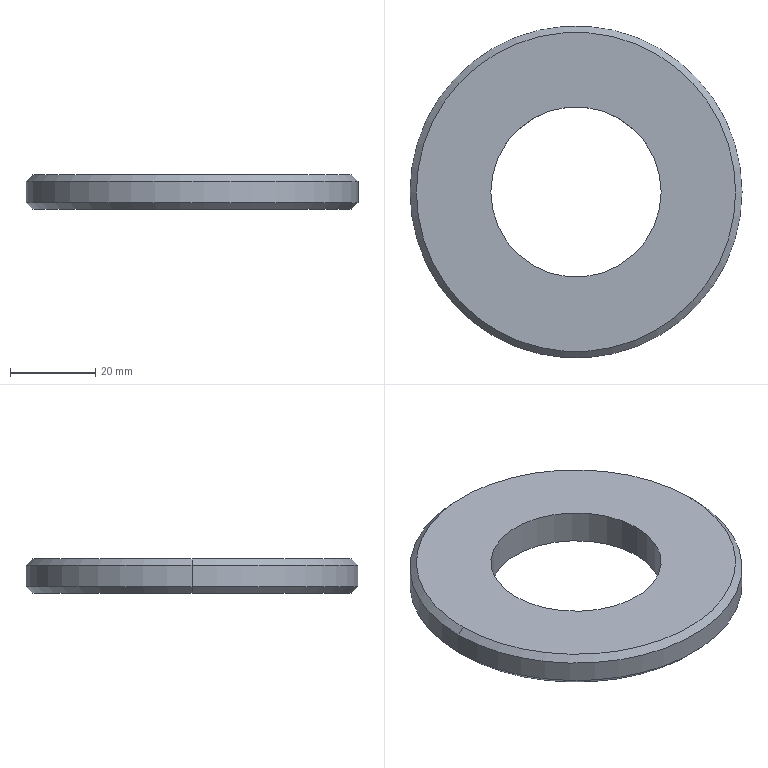Part | Creo | features DATUM PLANE 3, CHAMFER 1, COORDINATE SYSTEM 1, CURVE 1, PROTRUSION 1 | 1 solid | 10 faces | box 78 x 78 x 8 mm | volume 27630 mm3 | cylinder 4 | cone 4 | plane 2 | commonest cylinder face diameters 40 x2 78 x2
STEP:
#1=CARTESIAN_POINT('',(0.,0.,0.));
#2=DIRECTION('',(0.,0.,1.));
#3=DIRECTION('',(1.,0.,0.));
#4=AXIS2_PLACEMENT_3D('',#1,#2,#3);
#5=CARTESIAN_POINT('',(-37.5,0.,0.));
#6=VERTEX_POINT('',#5);
#7=CARTESIAN_POINT('',(37.5,0.,0.));
#8=VERTEX_POINT('',#7);
#9=CARTESIAN_POINT('',(0.,0.,0.));
#10=DIRECTION('',(0.,0.,-1.));
#11=DIRECTION('',(-1.,0.,0.));
#12=AXIS2_PLACEMENT_3D('',#9,#10,#11);
#13=CIRCLE('',#12,37.5);
#14=EDGE_CURVE('',#6,#8,#13,.T.);
#15=ORIENTED_EDGE('',*,*,#14,.F.);
#16=CARTESIAN_POINT('',(0.,0.,0.));
#17=DIRECTION('',(0.,0.,-1.));
#18=DIRECTION('',(1.,0.,0.));
#19=AXIS2_PLACEMENT_3D('',#16,#17,#18);
#20=CIRCLE('',#19,37.5);
#21=EDGE_CURVE('',#8,#6,#20,.T.);
#22=ORIENTED_EDGE('',*,*,#21,.F.);
#23=EDGE_LOOP('',(#15,#22));
#24=FACE_OUTER_BOUND('',#23,.F.);
#25=CARTESIAN_POINT('',(20.,0.,0.));
#26=VERTEX_POINT('',#25);
#27=CARTESIAN_POINT('',(-20.,0.,0.));
#28=VERTEX_POINT('',#27);
#29=CARTESIAN_POINT('',(0.,0.,0.));
#30=DIRECTION('',(0.,0.,-1.));
#31=DIRECTION('',(1.,0.,0.));
#32=AXIS2_PLACEMENT_3D('',#29,#30,#31);
#33=CIRCLE('',#32,20.);
#34=EDGE_CURVE('',#26,#28,#33,.T.);
#35=ORIENTED_EDGE('',*,*,#34,.T.);
#36=CARTESIAN_POINT('',(0.,0.,0.));
#37=DIRECTION('',(0.,0.,-1.));
#38=DIRECTION('',(-1.,0.,0.));
#39=AXIS2_PLACEMENT_3D('',#36,#37,#38);
#40=CIRCLE('',#39,20.);
#41=EDGE_CURVE('',#28,#26,#40,.T.);
#42=ORIENTED_EDGE('',*,*,#41,.T.);
#43=EDGE_LOOP('',(#35,#42));
#44=FACE_BOUND('',#43,.F.);
#45=CARTESIAN_POINT('',(0.,0.,0.));
#46=DIRECTION('',(0.,0.,1.));
#47=DIRECTION('',(1.,0.,0.));
#48=AXIS2_PLACEMENT_3D('',#45,#46,#47);
#49=PLANE('',#48);
#50=ADVANCED_FACE('',(#24,#44),#49,.F.);
#51=ORIENTED_EDGE('',*,*,#34,.F.);
#52=CARTESIAN_POINT('',(20.,0.,8.));
#53=VERTEX_POINT('',#52);
#54=CARTESIAN_POINT('',(20.,0.,0.));
#55=DIRECTION('',(0.,0.,1.));
#56=VECTOR('',#55,8.);
#57=LINE('',#54,#56);
#58=EDGE_CURVE('',#26,#53,#57,.T.);
#59=ORIENTED_EDGE('',*,*,#58,.T.);
#60=CARTESIAN_POINT('',(-20.,0.,8.));
#61=VERTEX_POINT('',#60);
#62=CARTESIAN_POINT('',(0.,0.,8.));
#63=DIRECTION('',(0.,0.,-1.));
#64=DIRECTION('',(1.,0.,0.));
#65=AXIS2_PLACEMENT_3D('',#62,#63,#64);
#66=CIRCLE('',#65,20.);
#67=EDGE_CURVE('',#53,#61,#66,.T.);
#68=ORIENTED_EDGE('',*,*,#67,.T.);
#69=CARTESIAN_POINT('',(-20.,0.,0.));
#70=DIRECTION('',(0.,0.,1.));
#71=VECTOR('',#70,8.);
#72=LINE('',#69,#71);
#73=EDGE_CURVE('',#28,#61,#72,.T.);
#74=ORIENTED_EDGE('',*,*,#73,.F.);
#75=EDGE_LOOP('',(#51,#59,#68,#74));
#76=FACE_OUTER_BOUND('',#75,.F.);
#77=CARTESIAN_POINT('',(0.,0.,0.));
#78=DIRECTION('',(0.,0.,1.));
#79=DIRECTION('',(1.,0.,0.));
#80=AXIS2_PLACEMENT_3D('',#77,#78,#79);
#81=CYLINDRICAL_SURFACE('',#80,20.);
#82=ADVANCED_FACE('',(#76),#81,.F.);
#83=ORIENTED_EDGE('',*,*,#41,.F.);
#84=ORIENTED_EDGE('',*,*,#73,.T.);
#85=CARTESIAN_POINT('',(0.,0.,8.));
#86=DIRECTION('',(0.,0.,-1.));
#87=DIRECTION('',(-1.,0.,0.));
#88=AXIS2_PLACEMENT_3D('',#85,#86,#87);
#89=CIRCLE('',#88,20.);
#90=EDGE_CURVE('',#61,#53,#89,.T.);
#91=ORIENTED_EDGE('',*,*,#90,.T.);
#92=ORIENTED_EDGE('',*,*,#58,.F.);
#93=EDGE_LOOP('',(#83,#84,#91,#92));
#94=FACE_OUTER_BOUND('',#93,.F.);
#95=CARTESIAN_POINT('',(0.,0.,0.));
#96=DIRECTION('',(0.,0.,1.));
#97=DIRECTION('',(1.,0.,0.));
#98=AXIS2_PLACEMENT_3D('',#95,#96,#97);
#99=CYLINDRICAL_SURFACE('',#98,20.);
#100=ADVANCED_FACE('',(#94),#99,.F.);
#101=CARTESIAN_POINT('',(37.5,0.,8.));
#102=VERTEX_POINT('',#101);
#103=CARTESIAN_POINT('',(-37.5,0.,8.));
#104=VERTEX_POINT('',#103);
#105=CARTESIAN_POINT('',(0.,0.,8.));
#106=DIRECTION('',(0.,0.,1.));
#107=DIRECTION('',(1.,0.,0.));
#108=AXIS2_PLACEMENT_3D('',#105,#106,#107);
#109=CIRCLE('',#108,37.5);
#110=EDGE_CURVE('',#102,#104,#109,.T.);
#111=ORIENTED_EDGE('',*,*,#110,.F.);
#112=CARTESIAN_POINT('',(0.,0.,8.));
#113=DIRECTION('',(0.,0.,1.));
#114=DIRECTION('',(-1.,0.,0.));
#115=AXIS2_PLACEMENT_3D('',#112,#113,#114);
#116=CIRCLE('',#115,37.5);
#117=EDGE_CURVE('',#104,#102,#116,.T.);
#118=ORIENTED_EDGE('',*,*,#117,.F.);
#119=EDGE_LOOP('',(#111,#118));
#120=FACE_OUTER_BOUND('',#119,.F.);
#121=ORIENTED_EDGE('',*,*,#67,.F.);
#122=ORIENTED_EDGE('',*,*,#90,.F.);
#123=EDGE_LOOP('',(#121,#122));
#124=FACE_BOUND('',#123,.F.);
#125=CARTESIAN_POINT('',(0.,0.,8.));
#126=DIRECTION('',(0.,0.,1.));
#127=DIRECTION('',(1.,0.,0.));
#128=AXIS2_PLACEMENT_3D('',#125,#126,#127);
#129=PLANE('',#128);
#130=ADVANCED_FACE('',(#120,#124),#129,.T.);
#131=ORIENTED_EDGE('',*,*,#110,.T.);
#132=CARTESIAN_POINT('',(-39.,0.,6.5));
#133=VERTEX_POINT('',#132);
#134=CARTESIAN_POINT('',(-37.5,-0.000000005,8.));
#135=DIRECTION('',(-0.7071,0.000000001,-0.7071));
#136=VECTOR('',#135,2.121);
#137=LINE('',#134,#136);
#138=EDGE_CURVE('',#104,#133,#137,.T.);
#139=ORIENTED_EDGE('',*,*,#138,.T.);
#140=CARTESIAN_POINT('',(39.,0.,6.5));
#141=VERTEX_POINT('',#140);
#142=CARTESIAN_POINT('',(0.,0.,6.5));
#143=DIRECTION('',(0.,0.,1.));
#144=DIRECTION('',(1.,0.,0.));
#145=AXIS2_PLACEMENT_3D('',#142,#143,#144);
#146=CIRCLE('',#145,39.);
#147=EDGE_CURVE('',#141,#133,#146,.T.);
#148=ORIENTED_EDGE('',*,*,#147,.F.);
#149=CARTESIAN_POINT('',(37.5,0.000000005,8.));
#150=DIRECTION('',(0.7071,-0.000000001,-0.7071));
#151=VECTOR('',#150,2.121);
#152=LINE('',#149,#151);
#153=EDGE_CURVE('',#102,#141,#152,.T.);
#154=ORIENTED_EDGE('',*,*,#153,.F.);
#155=EDGE_LOOP('',(#131,#139,#148,#154));
#156=FACE_OUTER_BOUND('',#155,.F.);
#157=CARTESIAN_POINT('',(0.,0.,7.25));
#158=DIRECTION('',(0.,0.,-1.));
#159=DIRECTION('',(0.,-1.,0.));
#160=AXIS2_PLACEMENT_3D('',#157,#158,#159);
#161=CONICAL_SURFACE('',#160,38.25,45.);
#162=ADVANCED_FACE('',(#156),#161,.T.);
#163=ORIENTED_EDGE('',*,*,#117,.T.);
#164=ORIENTED_EDGE('',*,*,#153,.T.);
#165=CARTESIAN_POINT('',(0.,0.,6.5));
#166=DIRECTION('',(0.,0.,1.));
#167=DIRECTION('',(-1.,0.,0.));
#168=AXIS2_PLACEMENT_3D('',#165,#166,#167);
#169=CIRCLE('',#168,39.);
#170=EDGE_CURVE('',#133,#141,#169,.T.);
#171=ORIENTED_EDGE('',*,*,#170,.F.);
#172=ORIENTED_EDGE('',*,*,#138,.F.);
#173=EDGE_LOOP('',(#163,#164,#171,#172));
#174=FACE_OUTER_BOUND('',#173,.F.);
#175=CARTESIAN_POINT('',(0.,0.,7.25));
#176=DIRECTION('',(0.,0.,-1.));
#177=DIRECTION('',(0.,-1.,0.));
#178=AXIS2_PLACEMENT_3D('',#175,#176,#177);
#179=CONICAL_SURFACE('',#178,38.25,45.);
#180=ADVANCED_FACE('',(#174),#179,.T.);
#181=ORIENTED_EDGE('',*,*,#170,.T.);
#182=CARTESIAN_POINT('',(39.,0.,1.5));
#183=VERTEX_POINT('',#182);
#184=CARTESIAN_POINT('',(39.,0.000000004,1.5));
#185=DIRECTION('',(0.,0.,1.));
#186=VECTOR('',#185,5.);
#187=LINE('',#184,#186);
#188=EDGE_CURVE('',#183,#141,#187,.T.);
#189=ORIENTED_EDGE('',*,*,#188,.F.);
#190=CARTESIAN_POINT('',(-39.,0.,1.5));
#191=VERTEX_POINT('',#190);
#192=CARTESIAN_POINT('',(0.,0.,1.5));
#193=DIRECTION('',(0.,0.,-1.));
#194=DIRECTION('',(1.,0.,0.));
#195=AXIS2_PLACEMENT_3D('',#192,#193,#194);
#196=CIRCLE('',#195,39.);
#197=EDGE_CURVE('',#183,#191,#196,.T.);
#198=ORIENTED_EDGE('',*,*,#197,.T.);
#199=CARTESIAN_POINT('',(-39.,-0.000000004,1.5));
#200=DIRECTION('',(0.,0.,1.));
#201=VECTOR('',#200,5.);
#202=LINE('',#199,#201);
#203=EDGE_CURVE('',#191,#133,#202,.T.);
#204=ORIENTED_EDGE('',*,*,#203,.T.);
#205=EDGE_LOOP('',(#181,#189,#198,#204));
#206=FACE_OUTER_BOUND('',#205,.F.);
#207=CARTESIAN_POINT('',(0.,0.,0.));
#208=DIRECTION('',(0.,0.,1.));
#209=DIRECTION('',(1.,0.,0.));
#210=AXIS2_PLACEMENT_3D('',#207,#208,#209);
#211=CYLINDRICAL_SURFACE('',#210,39.);
#212=ADVANCED_FACE('',(#206),#211,.T.);
#213=ORIENTED_EDGE('',*,*,#147,.T.);
#214=ORIENTED_EDGE('',*,*,#203,.F.);
#215=CARTESIAN_POINT('',(0.,0.,1.5));
#216=DIRECTION('',(0.,0.,-1.));
#217=DIRECTION('',(-1.,0.,0.));
#218=AXIS2_PLACEMENT_3D('',#215,#216,#217);
#219=CIRCLE('',#218,39.);
#220=EDGE_CURVE('',#191,#183,#219,.T.);
#221=ORIENTED_EDGE('',*,*,#220,.T.);
#222=ORIENTED_EDGE('',*,*,#188,.T.);
#223=EDGE_LOOP('',(#213,#214,#221,#222));
#224=FACE_OUTER_BOUND('',#223,.F.);
#225=CARTESIAN_POINT('',(0.,0.,0.));
#226=DIRECTION('',(0.,0.,1.));
#227=DIRECTION('',(1.,0.,0.));
#228=AXIS2_PLACEMENT_3D('',#225,#226,#227);
#229=CYLINDRICAL_SURFACE('',#228,39.);
#230=ADVANCED_FACE('',(#224),#229,.T.);
#231=ORIENTED_EDGE('',*,*,#14,.T.);
#232=CARTESIAN_POINT('',(37.5,0.000000005,0.));
#233=DIRECTION('',(0.7071,-0.000000001,0.7071));
#234=VECTOR('',#233,2.121);
#235=LINE('',#232,#234);
#236=EDGE_CURVE('',#8,#183,#235,.T.);
#237=ORIENTED_EDGE('',*,*,#236,.T.);
#238=ORIENTED_EDGE('',*,*,#220,.F.);
#239=CARTESIAN_POINT('',(-37.5,-0.000000005,0.));
#240=DIRECTION('',(-0.7071,0.000000001,0.7071));
#241=VECTOR('',#240,2.121);
#242=LINE('',#239,#241);
#243=EDGE_CURVE('',#6,#191,#242,.T.);
#244=ORIENTED_EDGE('',*,*,#243,.F.);
#245=EDGE_LOOP('',(#231,#237,#238,#244));
#246=FACE_OUTER_BOUND('',#245,.F.);
#247=CARTESIAN_POINT('',(0.,0.,0.75));
#248=DIRECTION('',(0.,0.,1.));
#249=DIRECTION('',(0.,-1.,0.));
#250=AXIS2_PLACEMENT_3D('',#247,#248,#249);
#251=CONICAL_SURFACE('',#250,38.25,45.);
#252=ADVANCED_FACE('',(#246),#251,.T.);
#253=ORIENTED_EDGE('',*,*,#21,.T.);
#254=ORIENTED_EDGE('',*,*,#243,.T.);
#255=ORIENTED_EDGE('',*,*,#197,.F.);
#256=ORIENTED_EDGE('',*,*,#236,.F.);
#257=EDGE_LOOP('',(#253,#254,#255,#256));
#258=FACE_OUTER_BOUND('',#257,.F.);
#259=CARTESIAN_POINT('',(0.,0.,0.75));
#260=DIRECTION('',(0.,0.,1.));
#261=DIRECTION('',(0.,-1.,0.));
#262=AXIS2_PLACEMENT_3D('',#259,#260,#261);
#263=CONICAL_SURFACE('',#262,38.25,45.);
#264=ADVANCED_FACE('',(#258),#263,.T.);
#265=CLOSED_SHELL('',(#50,#82,#100,#130,#162,#180,#212,#230,#252,#264));
#266=MANIFOLD_SOLID_BREP('',#265);
#267=(LENGTH_UNIT()NAMED_UNIT(*)SI_UNIT(.MILLI.,.METRE.));
#268=UNCERTAINTY_MEASURE_WITH_UNIT(LENGTH_MEASURE(0.01106),#267,'','');
#269=(NAMED_UNIT(*)PLANE_ANGLE_UNIT()SI_UNIT($,.RADIAN.));
#270=PLANE_ANGLE_MEASURE_WITH_UNIT(PLANE_ANGLE_MEASURE(0.01745),#269);
#271=(CONVERSION_BASED_UNIT('DEGREE',#270)NAMED_UNIT(*)PLANE_ANGLE_UNIT());
#272=(NAMED_UNIT(*)SI_UNIT($,.STERADIAN.)SOLID_ANGLE_UNIT());
#273=(GEOMETRIC_REPRESENTATION_CONTEXT(3)GLOBAL_UNCERTAINTY_ASSIGNED_CONTEXT((#268))GLOBAL_UNIT_ASSIGNED_CONTEXT((#267,#271,#272))REPRESENTATION_CONTEXT('',''));
#274=ADVANCED_BREP_SHAPE_REPRESENTATION('',(#4,#266),#273);